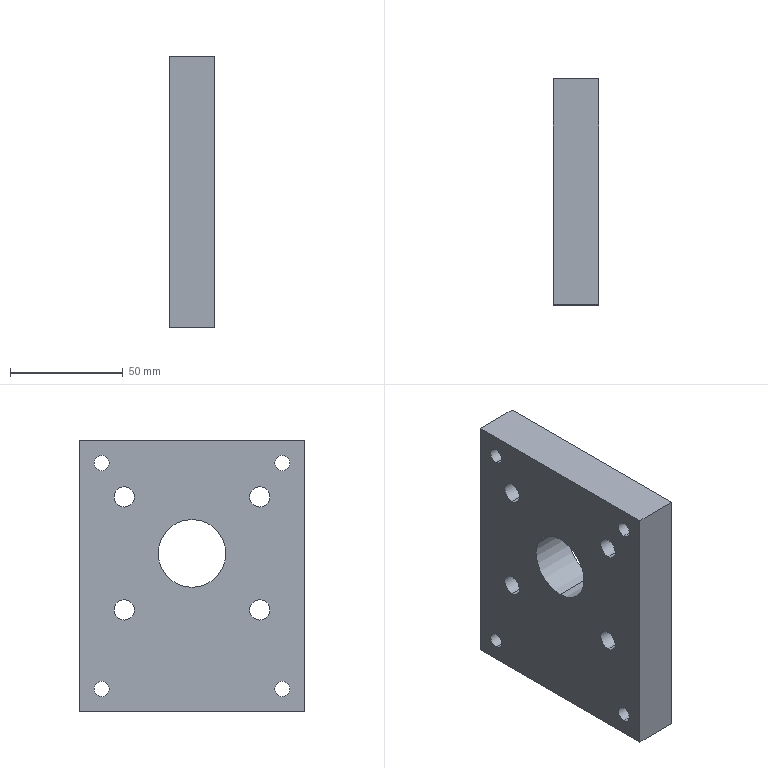Part | SolidWorks | features HoleWzd 2, Extrusion 1, ICE 1 | 1 solid | 36 faces | box 20 x 100 x 120 mm | volume 213797 mm3 | cylinder 26 | plane 10 | commonest cylinder face diameters 6.8 x8 9 x8 15 x8 30 x2
STEP:
#1=CARTESIAN_POINT('',(0.,40.,53.4));
#2=VERTEX_POINT('',#1);
#3=CARTESIAN_POINT('',(0.,40.,46.6));
#4=VERTEX_POINT('',#3);
#5=CARTESIAN_POINT('',(0.,40.,50.));
#6=DIRECTION('',(1.,0.,0.));
#7=DIRECTION('',(0.,0.,-1.));
#8=AXIS2_PLACEMENT_3D('',#5,#6,#7);
#9=CIRCLE('',#8,3.4);
#10=EDGE_CURVE('',#2,#4,#9,.T.);
#11=ORIENTED_EDGE('',*,*,#10,.F.);
#12=CARTESIAN_POINT('',(20.,40.,53.4));
#13=VERTEX_POINT('',#12);
#14=CARTESIAN_POINT('',(20.,40.,53.4));
#15=DIRECTION('',(1.,0.,0.));
#16=VECTOR('',#15,1000.);
#17=LINE('',#14,#16);
#18=EDGE_CURVE('',#2,#13,#17,.T.);
#19=ORIENTED_EDGE('',*,*,#18,.T.);
#20=CARTESIAN_POINT('',(20.,40.,46.6));
#21=VERTEX_POINT('',#20);
#22=CARTESIAN_POINT('',(20.,40.,50.));
#23=DIRECTION('',(1.,0.,0.));
#24=DIRECTION('',(0.,0.,-1.));
#25=AXIS2_PLACEMENT_3D('',#22,#23,#24);
#26=CIRCLE('',#25,3.4);
#27=EDGE_CURVE('',#13,#21,#26,.T.);
#28=ORIENTED_EDGE('',*,*,#27,.T.);
#29=CARTESIAN_POINT('',(20.,40.,46.6));
#30=DIRECTION('',(1.,0.,0.));
#31=VECTOR('',#30,1000.);
#32=LINE('',#29,#31);
#33=EDGE_CURVE('',#4,#21,#32,.T.);
#34=ORIENTED_EDGE('',*,*,#33,.F.);
#35=EDGE_LOOP('',(#11,#19,#28,#34));
#36=FACE_OUTER_BOUND('',#35,.T.);
#37=CARTESIAN_POINT('',(20.,40.,50.));
#38=DIRECTION('',(1.,0.,0.));
#39=DIRECTION('',(0.,0.,-1.));
#40=AXIS2_PLACEMENT_3D('',#37,#38,#39);
#41=CYLINDRICAL_SURFACE('',#40,3.4);
#42=ADVANCED_FACE('',(#36),#41,.F.);
#43=CARTESIAN_POINT('',(0.,-40.,53.4));
#44=VERTEX_POINT('',#43);
#45=CARTESIAN_POINT('',(0.,-40.,46.6));
#46=VERTEX_POINT('',#45);
#47=CARTESIAN_POINT('',(0.,-40.,50.));
#48=DIRECTION('',(1.,0.,0.));
#49=DIRECTION('',(0.,0.,-1.));
#50=AXIS2_PLACEMENT_3D('',#47,#48,#49);
#51=CIRCLE('',#50,3.4);
#52=EDGE_CURVE('',#44,#46,#51,.T.);
#53=ORIENTED_EDGE('',*,*,#52,.F.);
#54=CARTESIAN_POINT('',(20.,-40.,53.4));
#55=VERTEX_POINT('',#54);
#56=CARTESIAN_POINT('',(20.,-40.,53.4));
#57=DIRECTION('',(1.,0.,0.));
#58=VECTOR('',#57,1000.);
#59=LINE('',#56,#58);
#60=EDGE_CURVE('',#44,#55,#59,.T.);
#61=ORIENTED_EDGE('',*,*,#60,.T.);
#62=CARTESIAN_POINT('',(20.,-40.,46.6));
#63=VERTEX_POINT('',#62);
#64=CARTESIAN_POINT('',(20.,-40.,50.));
#65=DIRECTION('',(1.,0.,0.));
#66=DIRECTION('',(0.,0.,-1.));
#67=AXIS2_PLACEMENT_3D('',#64,#65,#66);
#68=CIRCLE('',#67,3.4);
#69=EDGE_CURVE('',#55,#63,#68,.T.);
#70=ORIENTED_EDGE('',*,*,#69,.T.);
#71=CARTESIAN_POINT('',(20.,-40.,46.6));
#72=DIRECTION('',(1.,0.,0.));
#73=VECTOR('',#72,1000.);
#74=LINE('',#71,#73);
#75=EDGE_CURVE('',#46,#63,#74,.T.);
#76=ORIENTED_EDGE('',*,*,#75,.F.);
#77=EDGE_LOOP('',(#53,#61,#70,#76));
#78=FACE_OUTER_BOUND('',#77,.T.);
#79=CARTESIAN_POINT('',(20.,-40.,50.));
#80=DIRECTION('',(1.,0.,0.));
#81=DIRECTION('',(0.,0.,-1.));
#82=AXIS2_PLACEMENT_3D('',#79,#80,#81);
#83=CYLINDRICAL_SURFACE('',#82,3.4);
#84=ADVANCED_FACE('',(#78),#83,.F.);
#85=CARTESIAN_POINT('',(0.,-40.,-46.6));
#86=VERTEX_POINT('',#85);
#87=CARTESIAN_POINT('',(0.,-40.,-53.4));
#88=VERTEX_POINT('',#87);
#89=CARTESIAN_POINT('',(0.,-40.,-50.));
#90=DIRECTION('',(1.,0.,0.));
#91=DIRECTION('',(0.,0.,-1.));
#92=AXIS2_PLACEMENT_3D('',#89,#90,#91);
#93=CIRCLE('',#92,3.4);
#94=EDGE_CURVE('',#86,#88,#93,.T.);
#95=ORIENTED_EDGE('',*,*,#94,.F.);
#96=CARTESIAN_POINT('',(20.,-40.,-46.6));
#97=VERTEX_POINT('',#96);
#98=CARTESIAN_POINT('',(20.,-40.,-46.6));
#99=DIRECTION('',(1.,0.,0.));
#100=VECTOR('',#99,1000.);
#101=LINE('',#98,#100);
#102=EDGE_CURVE('',#86,#97,#101,.T.);
#103=ORIENTED_EDGE('',*,*,#102,.T.);
#104=CARTESIAN_POINT('',(20.,-40.,-53.4));
#105=VERTEX_POINT('',#104);
#106=CARTESIAN_POINT('',(20.,-40.,-50.));
#107=DIRECTION('',(1.,0.,0.));
#108=DIRECTION('',(0.,0.,-1.));
#109=AXIS2_PLACEMENT_3D('',#106,#107,#108);
#110=CIRCLE('',#109,3.4);
#111=EDGE_CURVE('',#97,#105,#110,.T.);
#112=ORIENTED_EDGE('',*,*,#111,.T.);
#113=CARTESIAN_POINT('',(20.,-40.,-53.4));
#114=DIRECTION('',(1.,0.,0.));
#115=VECTOR('',#114,1000.);
#116=LINE('',#113,#115);
#117=EDGE_CURVE('',#88,#105,#116,.T.);
#118=ORIENTED_EDGE('',*,*,#117,.F.);
#119=EDGE_LOOP('',(#95,#103,#112,#118));
#120=FACE_OUTER_BOUND('',#119,.T.);
#121=CARTESIAN_POINT('',(20.,-40.,-50.));
#122=DIRECTION('',(1.,0.,0.));
#123=DIRECTION('',(0.,0.,-1.));
#124=AXIS2_PLACEMENT_3D('',#121,#122,#123);
#125=CYLINDRICAL_SURFACE('',#124,3.4);
#126=ADVANCED_FACE('',(#120),#125,.F.);
#127=CARTESIAN_POINT('',(0.,40.,-46.6));
#128=VERTEX_POINT('',#127);
#129=CARTESIAN_POINT('',(0.,40.,-53.4));
#130=VERTEX_POINT('',#129);
#131=CARTESIAN_POINT('',(0.,40.,-50.));
#132=DIRECTION('',(1.,0.,0.));
#133=DIRECTION('',(0.,0.,-1.));
#134=AXIS2_PLACEMENT_3D('',#131,#132,#133);
#135=CIRCLE('',#134,3.4);
#136=EDGE_CURVE('',#128,#130,#135,.T.);
#137=ORIENTED_EDGE('',*,*,#136,.F.);
#138=CARTESIAN_POINT('',(20.,40.,-46.6));
#139=VERTEX_POINT('',#138);
#140=CARTESIAN_POINT('',(20.,40.,-46.6));
#141=DIRECTION('',(1.,0.,0.));
#142=VECTOR('',#141,1000.);
#143=LINE('',#140,#142);
#144=EDGE_CURVE('',#128,#139,#143,.T.);
#145=ORIENTED_EDGE('',*,*,#144,.T.);
#146=CARTESIAN_POINT('',(20.,40.,-53.4));
#147=VERTEX_POINT('',#146);
#148=CARTESIAN_POINT('',(20.,40.,-50.));
#149=DIRECTION('',(1.,0.,0.));
#150=DIRECTION('',(0.,0.,-1.));
#151=AXIS2_PLACEMENT_3D('',#148,#149,#150);
#152=CIRCLE('',#151,3.4);
#153=EDGE_CURVE('',#139,#147,#152,.T.);
#154=ORIENTED_EDGE('',*,*,#153,.T.);
#155=CARTESIAN_POINT('',(20.,40.,-53.4));
#156=DIRECTION('',(1.,0.,0.));
#157=VECTOR('',#156,1000.);
#158=LINE('',#155,#157);
#159=EDGE_CURVE('',#130,#147,#158,.T.);
#160=ORIENTED_EDGE('',*,*,#159,.F.);
#161=EDGE_LOOP('',(#137,#145,#154,#160));
#162=FACE_OUTER_BOUND('',#161,.T.);
#163=CARTESIAN_POINT('',(20.,40.,-50.));
#164=DIRECTION('',(1.,0.,0.));
#165=DIRECTION('',(0.,0.,-1.));
#166=AXIS2_PLACEMENT_3D('',#163,#164,#165);
#167=CYLINDRICAL_SURFACE('',#166,3.4);
#168=ADVANCED_FACE('',(#162),#167,.F.);
#169=CARTESIAN_POINT('',(0.,0.,25.));
#170=VERTEX_POINT('',#169);
#171=CARTESIAN_POINT('',(0.,0.,-5.));
#172=VERTEX_POINT('',#171);
#173=CARTESIAN_POINT('',(0.,0.,10.));
#174=DIRECTION('',(1.,0.,0.));
#175=DIRECTION('',(0.,0.,-1.));
#176=AXIS2_PLACEMENT_3D('',#173,#174,#175);
#177=CIRCLE('',#176,15.);
#178=EDGE_CURVE('',#170,#172,#177,.T.);
#179=ORIENTED_EDGE('',*,*,#178,.F.);
#180=CARTESIAN_POINT('',(20.,0.,25.));
#181=VERTEX_POINT('',#180);
#182=CARTESIAN_POINT('',(0.,0.,25.));
#183=DIRECTION('',(1.,0.,0.));
#184=VECTOR('',#183,1000.);
#185=LINE('',#182,#184);
#186=EDGE_CURVE('',#170,#181,#185,.T.);
#187=ORIENTED_EDGE('',*,*,#186,.T.);
#188=CARTESIAN_POINT('',(20.,0.,-5.));
#189=VERTEX_POINT('',#188);
#190=CARTESIAN_POINT('',(20.,0.,10.));
#191=DIRECTION('',(1.,0.,0.));
#192=DIRECTION('',(0.,0.,-1.));
#193=AXIS2_PLACEMENT_3D('',#190,#191,#192);
#194=CIRCLE('',#193,15.);
#195=EDGE_CURVE('',#181,#189,#194,.T.);
#196=ORIENTED_EDGE('',*,*,#195,.T.);
#197=CARTESIAN_POINT('',(0.,0.,-5.));
#198=DIRECTION('',(1.,0.,0.));
#199=VECTOR('',#198,1000.);
#200=LINE('',#197,#199);
#201=EDGE_CURVE('',#172,#189,#200,.T.);
#202=ORIENTED_EDGE('',*,*,#201,.F.);
#203=EDGE_LOOP('',(#179,#187,#196,#202));
#204=FACE_OUTER_BOUND('',#203,.T.);
#205=CARTESIAN_POINT('',(0.,0.,10.));
#206=DIRECTION('',(1.,0.,0.));
#207=DIRECTION('',(0.,0.,-1.));
#208=AXIS2_PLACEMENT_3D('',#205,#206,#207);
#209=CYLINDRICAL_SURFACE('',#208,15.);
#210=ADVANCED_FACE('',(#204),#209,.F.);
#211=CARTESIAN_POINT('',(11.,30.,42.5));
#212=VERTEX_POINT('',#211);
#213=CARTESIAN_POINT('',(11.,30.,27.5));
#214=VERTEX_POINT('',#213);
#215=CARTESIAN_POINT('',(11.,30.,35.));
#216=DIRECTION('',(1.,0.,0.));
#217=DIRECTION('',(0.,0.,-1.));
#218=AXIS2_PLACEMENT_3D('',#215,#216,#217);
#219=CIRCLE('',#218,7.5);
#220=EDGE_CURVE('',#212,#214,#219,.T.);
#221=ORIENTED_EDGE('',*,*,#220,.F.);
#222=CARTESIAN_POINT('',(20.,30.,42.5));
#223=VERTEX_POINT('',#222);
#224=CARTESIAN_POINT('',(20.,30.,42.5));
#225=DIRECTION('',(1.,0.,0.));
#226=VECTOR('',#225,1000.);
#227=LINE('',#224,#226);
#228=EDGE_CURVE('',#212,#223,#227,.T.);
#229=ORIENTED_EDGE('',*,*,#228,.T.);
#230=CARTESIAN_POINT('',(20.,30.,27.5));
#231=VERTEX_POINT('',#230);
#232=CARTESIAN_POINT('',(20.,30.,35.));
#233=DIRECTION('',(1.,0.,0.));
#234=DIRECTION('',(0.,0.,-1.));
#235=AXIS2_PLACEMENT_3D('',#232,#233,#234);
#236=CIRCLE('',#235,7.5);
#237=EDGE_CURVE('',#223,#231,#236,.T.);
#238=ORIENTED_EDGE('',*,*,#237,.T.);
#239=CARTESIAN_POINT('',(20.,30.,27.5));
#240=DIRECTION('',(1.,0.,0.));
#241=VECTOR('',#240,1000.);
#242=LINE('',#239,#241);
#243=EDGE_CURVE('',#214,#231,#242,.T.);
#244=ORIENTED_EDGE('',*,*,#243,.F.);
#245=EDGE_LOOP('',(#221,#229,#238,#244));
#246=FACE_OUTER_BOUND('',#245,.T.);
#247=CARTESIAN_POINT('',(20.,30.,35.));
#248=DIRECTION('',(1.,0.,0.));
#249=DIRECTION('',(0.,0.,-1.));
#250=AXIS2_PLACEMENT_3D('',#247,#248,#249);
#251=CYLINDRICAL_SURFACE('',#250,7.5);
#252=ADVANCED_FACE('',(#246),#251,.F.);
#253=CARTESIAN_POINT('',(0.,30.,39.5));
#254=VERTEX_POINT('',#253);
#255=CARTESIAN_POINT('',(0.,30.,30.5));
#256=VERTEX_POINT('',#255);
#257=CARTESIAN_POINT('',(0.,30.,35.));
#258=DIRECTION('',(1.,0.,0.));
#259=DIRECTION('',(0.,0.,-1.));
#260=AXIS2_PLACEMENT_3D('',#257,#258,#259);
#261=CIRCLE('',#260,4.5);
#262=EDGE_CURVE('',#254,#256,#261,.T.);
#263=ORIENTED_EDGE('',*,*,#262,.F.);
#264=CARTESIAN_POINT('',(11.,30.,39.5));
#265=VERTEX_POINT('',#264);
#266=CARTESIAN_POINT('',(20.,30.,39.5));
#267=DIRECTION('',(1.,0.,0.));
#268=VECTOR('',#267,1000.);
#269=LINE('',#266,#268);
#270=EDGE_CURVE('',#254,#265,#269,.T.);
#271=ORIENTED_EDGE('',*,*,#270,.T.);
#272=CARTESIAN_POINT('',(11.,30.,30.5));
#273=VERTEX_POINT('',#272);
#274=CARTESIAN_POINT('',(11.,30.,35.));
#275=DIRECTION('',(1.,0.,0.));
#276=DIRECTION('',(0.,0.,-1.));
#277=AXIS2_PLACEMENT_3D('',#274,#275,#276);
#278=CIRCLE('',#277,4.5);
#279=EDGE_CURVE('',#265,#273,#278,.T.);
#280=ORIENTED_EDGE('',*,*,#279,.T.);
#281=CARTESIAN_POINT('',(20.,30.,30.5));
#282=DIRECTION('',(1.,0.,0.));
#283=VECTOR('',#282,1000.);
#284=LINE('',#281,#283);
#285=EDGE_CURVE('',#256,#273,#284,.T.);
#286=ORIENTED_EDGE('',*,*,#285,.F.);
#287=EDGE_LOOP('',(#263,#271,#280,#286));
#288=FACE_OUTER_BOUND('',#287,.T.);
#289=CARTESIAN_POINT('',(20.,30.,35.));
#290=DIRECTION('',(1.,0.,0.));
#291=DIRECTION('',(0.,0.,-1.));
#292=AXIS2_PLACEMENT_3D('',#289,#290,#291);
#293=CYLINDRICAL_SURFACE('',#292,4.5);
#294=ADVANCED_FACE('',(#288),#293,.F.);
#295=CARTESIAN_POINT('',(11.,30.,-7.5));
#296=VERTEX_POINT('',#295);
#297=CARTESIAN_POINT('',(11.,30.,-22.5));
#298=VERTEX_POINT('',#297);
#299=CARTESIAN_POINT('',(11.,30.,-15.));
#300=DIRECTION('',(1.,0.,0.));
#301=DIRECTION('',(0.,0.,-1.));
#302=AXIS2_PLACEMENT_3D('',#299,#300,#301);
#303=CIRCLE('',#302,7.5);
#304=EDGE_CURVE('',#296,#298,#303,.T.);
#305=ORIENTED_EDGE('',*,*,#304,.F.);
#306=CARTESIAN_POINT('',(20.,30.,-7.5));
#307=VERTEX_POINT('',#306);
#308=CARTESIAN_POINT('',(20.,30.,-7.5));
#309=DIRECTION('',(1.,0.,0.));
#310=VECTOR('',#309,1000.);
#311=LINE('',#308,#310);
#312=EDGE_CURVE('',#296,#307,#311,.T.);
#313=ORIENTED_EDGE('',*,*,#312,.T.);
#314=CARTESIAN_POINT('',(20.,30.,-22.5));
#315=VERTEX_POINT('',#314);
#316=CARTESIAN_POINT('',(20.,30.,-15.));
#317=DIRECTION('',(1.,0.,0.));
#318=DIRECTION('',(0.,0.,-1.));
#319=AXIS2_PLACEMENT_3D('',#316,#317,#318);
#320=CIRCLE('',#319,7.5);
#321=EDGE_CURVE('',#307,#315,#320,.T.);
#322=ORIENTED_EDGE('',*,*,#321,.T.);
#323=CARTESIAN_POINT('',(20.,30.,-22.5));
#324=DIRECTION('',(1.,0.,0.));
#325=VECTOR('',#324,1000.);
#326=LINE('',#323,#325);
#327=EDGE_CURVE('',#298,#315,#326,.T.);
#328=ORIENTED_EDGE('',*,*,#327,.F.);
#329=EDGE_LOOP('',(#305,#313,#322,#328));
#330=FACE_OUTER_BOUND('',#329,.T.);
#331=CARTESIAN_POINT('',(20.,30.,-15.));
#332=DIRECTION('',(1.,0.,0.));
#333=DIRECTION('',(0.,0.,-1.));
#334=AXIS2_PLACEMENT_3D('',#331,#332,#333);
#335=CYLINDRICAL_SURFACE('',#334,7.5);
#336=ADVANCED_FACE('',(#330),#335,.F.);
#337=CARTESIAN_POINT('',(0.,30.,-10.5));
#338=VERTEX_POINT('',#337);
#339=CARTESIAN_POINT('',(0.,30.,-19.5));
#340=VERTEX_POINT('',#339);
#341=CARTESIAN_POINT('',(0.,30.,-15.));
#342=DIRECTION('',(1.,0.,0.));
#343=DIRECTION('',(0.,0.,-1.));
#344=AXIS2_PLACEMENT_3D('',#341,#342,#343);
#345=CIRCLE('',#344,4.5);
#346=EDGE_CURVE('',#338,#340,#345,.T.);
#347=ORIENTED_EDGE('',*,*,#346,.F.);
#348=CARTESIAN_POINT('',(11.,30.,-10.5));
#349=VERTEX_POINT('',#348);
#350=CARTESIAN_POINT('',(20.,30.,-10.5));
#351=DIRECTION('',(1.,0.,0.));
#352=VECTOR('',#351,1000.);
#353=LINE('',#350,#352);
#354=EDGE_CURVE('',#338,#349,#353,.T.);
#355=ORIENTED_EDGE('',*,*,#354,.T.);
#356=CARTESIAN_POINT('',(11.,30.,-19.5));
#357=VERTEX_POINT('',#356);
#358=CARTESIAN_POINT('',(11.,30.,-15.));
#359=DIRECTION('',(1.,0.,0.));
#360=DIRECTION('',(0.,0.,-1.));
#361=AXIS2_PLACEMENT_3D('',#358,#359,#360);
#362=CIRCLE('',#361,4.5);
#363=EDGE_CURVE('',#349,#357,#362,.T.);
#364=ORIENTED_EDGE('',*,*,#363,.T.);
#365=CARTESIAN_POINT('',(20.,30.,-19.5));
#366=DIRECTION('',(1.,0.,0.));
#367=VECTOR('',#366,1000.);
#368=LINE('',#365,#367);
#369=EDGE_CURVE('',#340,#357,#368,.T.);
#370=ORIENTED_EDGE('',*,*,#369,.F.);
#371=EDGE_LOOP('',(#347,#355,#364,#370));
#372=FACE_OUTER_BOUND('',#371,.T.);
#373=CARTESIAN_POINT('',(20.,30.,-15.));
#374=DIRECTION('',(1.,0.,0.));
#375=DIRECTION('',(0.,0.,-1.));
#376=AXIS2_PLACEMENT_3D('',#373,#374,#375);
#377=CYLINDRICAL_SURFACE('',#376,4.5);
#378=ADVANCED_FACE('',(#372),#377,.F.);
#379=CARTESIAN_POINT('',(11.,-30.,42.5));
#380=VERTEX_POINT('',#379);
#381=CARTESIAN_POINT('',(11.,-30.,27.5));
#382=VERTEX_POINT('',#381);
#383=CARTESIAN_POINT('',(11.,-30.,35.));
#384=DIRECTION('',(1.,0.,0.));
#385=DIRECTION('',(0.,0.,-1.));
#386=AXIS2_PLACEMENT_3D('',#383,#384,#385);
#387=CIRCLE('',#386,7.5);
#388=EDGE_CURVE('',#380,#382,#387,.T.);
#389=ORIENTED_EDGE('',*,*,#388,.F.);
#390=CARTESIAN_POINT('',(20.,-30.,42.5));
#391=VERTEX_POINT('',#390);
#392=CARTESIAN_POINT('',(20.,-30.,42.5));
#393=DIRECTION('',(1.,0.,0.));
#394=VECTOR('',#393,1000.);
#395=LINE('',#392,#394);
#396=EDGE_CURVE('',#380,#391,#395,.T.);
#397=ORIENTED_EDGE('',*,*,#396,.T.);
#398=CARTESIAN_POINT('',(20.,-30.,27.5));
#399=VERTEX_POINT('',#398);
#400=CARTESIAN_POINT('',(20.,-30.,35.));
#401=DIRECTION('',(1.,0.,0.));
#402=DIRECTION('',(0.,0.,-1.));
#403=AXIS2_PLACEMENT_3D('',#400,#401,#402);
#404=CIRCLE('',#403,7.5);
#405=EDGE_CURVE('',#391,#399,#404,.T.);
#406=ORIENTED_EDGE('',*,*,#405,.T.);
#407=CARTESIAN_POINT('',(20.,-30.,27.5));
#408=DIRECTION('',(1.,0.,0.));
#409=VECTOR('',#408,1000.);
#410=LINE('',#407,#409);
#411=EDGE_CURVE('',#382,#399,#410,.T.);
#412=ORIENTED_EDGE('',*,*,#411,.F.);
#413=EDGE_LOOP('',(#389,#397,#406,#412));
#414=FACE_OUTER_BOUND('',#413,.T.);
#415=CARTESIAN_POINT('',(20.,-30.,35.));
#416=DIRECTION('',(1.,0.,0.));
#417=DIRECTION('',(0.,0.,-1.));
#418=AXIS2_PLACEMENT_3D('',#415,#416,#417);
#419=CYLINDRICAL_SURFACE('',#418,7.5);
#420=ADVANCED_FACE('',(#414),#419,.F.);
#421=CARTESIAN_POINT('',(0.,-30.,39.5));
#422=VERTEX_POINT('',#421);
#423=CARTESIAN_POINT('',(0.,-30.,30.5));
#424=VERTEX_POINT('',#423);
#425=CARTESIAN_POINT('',(0.,-30.,35.));
#426=DIRECTION('',(1.,0.,0.));
#427=DIRECTION('',(0.,0.,-1.));
#428=AXIS2_PLACEMENT_3D('',#425,#426,#427);
#429=CIRCLE('',#428,4.5);
#430=EDGE_CURVE('',#422,#424,#429,.T.);
#431=ORIENTED_EDGE('',*,*,#430,.F.);
#432=CARTESIAN_POINT('',(11.,-30.,39.5));
#433=VERTEX_POINT('',#432);
#434=CARTESIAN_POINT('',(20.,-30.,39.5));
#435=DIRECTION('',(1.,0.,0.));
#436=VECTOR('',#435,1000.);
#437=LINE('',#434,#436);
#438=EDGE_CURVE('',#422,#433,#437,.T.);
#439=ORIENTED_EDGE('',*,*,#438,.T.);
#440=CARTESIAN_POINT('',(11.,-30.,30.5));
#441=VERTEX_POINT('',#440);
#442=CARTESIAN_POINT('',(11.,-30.,35.));
#443=DIRECTION('',(1.,0.,0.));
#444=DIRECTION('',(0.,0.,-1.));
#445=AXIS2_PLACEMENT_3D('',#442,#443,#444);
#446=CIRCLE('',#445,4.5);
#447=EDGE_CURVE('',#433,#441,#446,.T.);
#448=ORIENTED_EDGE('',*,*,#447,.T.);
#449=CARTESIAN_POINT('',(20.,-30.,30.5));
#450=DIRECTION('',(1.,0.,0.));
#451=VECTOR('',#450,1000.);
#452=LINE('',#449,#451);
#453=EDGE_CURVE('',#424,#441,#452,.T.);
#454=ORIENTED_EDGE('',*,*,#453,.F.);
#455=EDGE_LOOP('',(#431,#439,#448,#454));
#456=FACE_OUTER_BOUND('',#455,.T.);
#457=CARTESIAN_POINT('',(20.,-30.,35.));
#458=DIRECTION('',(1.,0.,0.));
#459=DIRECTION('',(0.,0.,-1.));
#460=AXIS2_PLACEMENT_3D('',#457,#458,#459);
#461=CYLINDRICAL_SURFACE('',#460,4.5);
#462=ADVANCED_FACE('',(#456),#461,.F.);
#463=CARTESIAN_POINT('',(11.,-30.,-7.5));
#464=VERTEX_POINT('',#463);
#465=CARTESIAN_POINT('',(11.,-30.,-22.5));
#466=VERTEX_POINT('',#465);
#467=CARTESIAN_POINT('',(11.,-30.,-15.));
#468=DIRECTION('',(1.,0.,0.));
#469=DIRECTION('',(0.,0.,-1.));
#470=AXIS2_PLACEMENT_3D('',#467,#468,#469);
#471=CIRCLE('',#470,7.5);
#472=EDGE_CURVE('',#464,#466,#471,.T.);
#473=ORIENTED_EDGE('',*,*,#472,.F.);
#474=CARTESIAN_POINT('',(20.,-30.,-7.5));
#475=VERTEX_POINT('',#474);
#476=CARTESIAN_POINT('',(20.,-30.,-7.5));
#477=DIRECTION('',(1.,0.,0.));
#478=VECTOR('',#477,1000.);
#479=LINE('',#476,#478);
#480=EDGE_CURVE('',#464,#475,#479,.T.);
#481=ORIENTED_EDGE('',*,*,#480,.T.);
#482=CARTESIAN_POINT('',(20.,-30.,-22.5));
#483=VERTEX_POINT('',#482);
#484=CARTESIAN_POINT('',(20.,-30.,-15.));
#485=DIRECTION('',(1.,0.,0.));
#486=DIRECTION('',(0.,0.,-1.));
#487=AXIS2_PLACEMENT_3D('',#484,#485,#486);
#488=CIRCLE('',#487,7.5);
#489=EDGE_CURVE('',#475,#483,#488,.T.);
#490=ORIENTED_EDGE('',*,*,#489,.T.);
#491=CARTESIAN_POINT('',(20.,-30.,-22.5));
#492=DIRECTION('',(1.,0.,0.));
#493=VECTOR('',#492,1000.);
#494=LINE('',#491,#493);
#495=EDGE_CURVE('',#466,#483,#494,.T.);
#496=ORIENTED_EDGE('',*,*,#495,.F.);
#497=EDGE_LOOP('',(#473,#481,#490,#496));
#498=FACE_OUTER_BOUND('',#497,.T.);
#499=CARTESIAN_POINT('',(20.,-30.,-15.));
#500=DIRECTION('',(1.,0.,0.));
#501=DIRECTION('',(0.,0.,-1.));
#502=AXIS2_PLACEMENT_3D('',#499,#500,#501);
#503=CYLINDRICAL_SURFACE('',#502,7.5);
#504=ADVANCED_FACE('',(#498),#503,.F.);
#505=CARTESIAN_POINT('',(0.,-30.,-10.5));
#506=VERTEX_POINT('',#505);
#507=CARTESIAN_POINT('',(0.,-30.,-19.5));
#508=VERTEX_POINT('',#507);
#509=CARTESIAN_POINT('',(0.,-30.,-15.));
#510=DIRECTION('',(1.,0.,0.));
#511=DIRECTION('',(0.,0.,-1.));
#512=AXIS2_PLACEMENT_3D('',#509,#510,#511);
#513=CIRCLE('',#512,4.5);
#514=EDGE_CURVE('',#506,#508,#513,.T.);
#515=ORIENTED_EDGE('',*,*,#514,.F.);
#516=CARTESIAN_POINT('',(11.,-30.,-10.5));
#517=VERTEX_POINT('',#516);
#518=CARTESIAN_POINT('',(20.,-30.,-10.5));
#519=DIRECTION('',(1.,0.,0.));
#520=VECTOR('',#519,1000.);
#521=LINE('',#518,#520);
#522=EDGE_CURVE('',#506,#517,#521,.T.);
#523=ORIENTED_EDGE('',*,*,#522,.T.);
#524=CARTESIAN_POINT('',(11.,-30.,-19.5));
#525=VERTEX_POINT('',#524);
#526=CARTESIAN_POINT('',(11.,-30.,-15.));
#527=DIRECTION('',(1.,0.,0.));
#528=DIRECTION('',(0.,0.,-1.));
#529=AXIS2_PLACEMENT_3D('',#526,#527,#528);
#530=CIRCLE('',#529,4.5);
#531=EDGE_CURVE('',#517,#525,#530,.T.);
#532=ORIENTED_EDGE('',*,*,#531,.T.);
#533=CARTESIAN_POINT('',(20.,-30.,-19.5));
#534=DIRECTION('',(1.,0.,0.));
#535=VECTOR('',#534,1000.);
#536=LINE('',#533,#535);
#537=EDGE_CURVE('',#508,#525,#536,.T.);
#538=ORIENTED_EDGE('',*,*,#537,.F.);
#539=EDGE_LOOP('',(#515,#523,#532,#538));
#540=FACE_OUTER_BOUND('',#539,.T.);
#541=CARTESIAN_POINT('',(20.,-30.,-15.));
#542=DIRECTION('',(1.,0.,0.));
#543=DIRECTION('',(0.,0.,-1.));
#544=AXIS2_PLACEMENT_3D('',#541,#542,#543);
#545=CYLINDRICAL_SURFACE('',#544,4.5);
#546=ADVANCED_FACE('',(#540),#545,.F.);
#547=CARTESIAN_POINT('',(0.,-50.,-60.));
#548=VERTEX_POINT('',#547);
#549=CARTESIAN_POINT('',(0.,50.,-60.));
#550=VERTEX_POINT('',#549);
#551=CARTESIAN_POINT('',(0.,50.,-60.));
#552=DIRECTION('',(0.,1.,0.));
#553=VECTOR('',#552,1000.);
#554=LINE('',#551,#553);
#555=EDGE_CURVE('',#548,#550,#554,.T.);
#556=ORIENTED_EDGE('',*,*,#555,.T.);
#557=CARTESIAN_POINT('',(20.,50.,-60.));
#558=VERTEX_POINT('',#557);
#559=CARTESIAN_POINT('',(20.,50.,-60.));
#560=DIRECTION('',(-1.,0.,0.));
#561=VECTOR('',#560,1000.);
#562=LINE('',#559,#561);
#563=EDGE_CURVE('',#558,#550,#562,.T.);
#564=ORIENTED_EDGE('',*,*,#563,.F.);
#565=CARTESIAN_POINT('',(20.,-50.,-60.));
#566=VERTEX_POINT('',#565);
#567=CARTESIAN_POINT('',(20.,50.,-60.));
#568=DIRECTION('',(0.,1.,0.));
#569=VECTOR('',#568,1000.);
#570=LINE('',#567,#569);
#571=EDGE_CURVE('',#566,#558,#570,.T.);
#572=ORIENTED_EDGE('',*,*,#571,.F.);
#573=CARTESIAN_POINT('',(20.,-50.,-60.));
#574=DIRECTION('',(-1.,0.,0.));
#575=VECTOR('',#574,1000.);
#576=LINE('',#573,#575);
#577=EDGE_CURVE('',#566,#548,#576,.T.);
#578=ORIENTED_EDGE('',*,*,#577,.T.);
#579=EDGE_LOOP('',(#556,#564,#572,#578));
#580=FACE_OUTER_BOUND('',#579,.T.);
#581=CARTESIAN_POINT('',(20.,50.,-60.));
#582=DIRECTION('',(0.,0.,1.));
#583=DIRECTION('',(0.,-1.,0.));
#584=AXIS2_PLACEMENT_3D('',#581,#582,#583);
#585=PLANE('',#584);
#586=ADVANCED_FACE('',(#580),#585,.F.);
#587=CARTESIAN_POINT('',(0.,50.,60.));
#588=VERTEX_POINT('',#587);
#589=CARTESIAN_POINT('',(0.,50.,60.));
#590=DIRECTION('',(0.,0.,1.));
#591=VECTOR('',#590,1000.);
#592=LINE('',#589,#591);
#593=EDGE_CURVE('',#550,#588,#592,.T.);
#594=ORIENTED_EDGE('',*,*,#593,.T.);
#595=CARTESIAN_POINT('',(20.,50.,60.));
#596=VERTEX_POINT('',#595);
#597=CARTESIAN_POINT('',(20.,50.,60.));
#598=DIRECTION('',(-1.,0.,0.));
#599=VECTOR('',#598,1000.);
#600=LINE('',#597,#599);
#601=EDGE_CURVE('',#596,#588,#600,.T.);
#602=ORIENTED_EDGE('',*,*,#601,.F.);
#603=CARTESIAN_POINT('',(20.,50.,60.));
#604=DIRECTION('',(0.,0.,1.));
#605=VECTOR('',#604,1000.);
#606=LINE('',#603,#605);
#607=EDGE_CURVE('',#558,#596,#606,.T.);
#608=ORIENTED_EDGE('',*,*,#607,.F.);
#609=ORIENTED_EDGE('',*,*,#563,.T.);
#610=EDGE_LOOP('',(#594,#602,#608,#609));
#611=FACE_OUTER_BOUND('',#610,.T.);
#612=CARTESIAN_POINT('',(20.,50.,60.));
#613=DIRECTION('',(0.,-1.,0.));
#614=DIRECTION('',(0.,0.,-1.));
#615=AXIS2_PLACEMENT_3D('',#612,#613,#614);
#616=PLANE('',#615);
#617=ADVANCED_FACE('',(#611),#616,.F.);
#618=CARTESIAN_POINT('',(0.,-50.,60.));
#619=VERTEX_POINT('',#618);
#620=CARTESIAN_POINT('',(0.,50.,60.));
#621=DIRECTION('',(0.,-1.,0.));
#622=VECTOR('',#621,1000.);
#623=LINE('',#620,#622);
#624=EDGE_CURVE('',#588,#619,#623,.T.);
#625=ORIENTED_EDGE('',*,*,#624,.T.);
#626=CARTESIAN_POINT('',(20.,-50.,60.));
#627=VERTEX_POINT('',#626);
#628=CARTESIAN_POINT('',(20.,-50.,60.));
#629=DIRECTION('',(-1.,0.,0.));
#630=VECTOR('',#629,1000.);
#631=LINE('',#628,#630);
#632=EDGE_CURVE('',#627,#619,#631,.T.);
#633=ORIENTED_EDGE('',*,*,#632,.F.);
#634=CARTESIAN_POINT('',(20.,50.,60.));
#635=DIRECTION('',(0.,-1.,0.));
#636=VECTOR('',#635,1000.);
#637=LINE('',#634,#636);
#638=EDGE_CURVE('',#596,#627,#637,.T.);
#639=ORIENTED_EDGE('',*,*,#638,.F.);
#640=ORIENTED_EDGE('',*,*,#601,.T.);
#641=EDGE_LOOP('',(#625,#633,#639,#640));
#642=FACE_OUTER_BOUND('',#641,.T.);
#643=CARTESIAN_POINT('',(20.,50.,60.));
#644=DIRECTION('',(0.,0.,-1.));
#645=DIRECTION('',(0.,1.,0.));
#646=AXIS2_PLACEMENT_3D('',#643,#644,#645);
#647=PLANE('',#646);
#648=ADVANCED_FACE('',(#642),#647,.F.);
#649=CARTESIAN_POINT('',(0.,-50.,60.));
#650=DIRECTION('',(0.,0.,-1.));
#651=VECTOR('',#650,1000.);
#652=LINE('',#649,#651);
#653=EDGE_CURVE('',#619,#548,#652,.T.);
#654=ORIENTED_EDGE('',*,*,#653,.T.);
#655=ORIENTED_EDGE('',*,*,#577,.F.);
#656=CARTESIAN_POINT('',(20.,-50.,60.));
#657=DIRECTION('',(0.,0.,-1.));
#658=VECTOR('',#657,1000.);
#659=LINE('',#656,#658);
#660=EDGE_CURVE('',#627,#566,#659,.T.);
#661=ORIENTED_EDGE('',*,*,#660,.F.);
#662=ORIENTED_EDGE('',*,*,#632,.T.);
#663=EDGE_LOOP('',(#654,#655,#661,#662));
#664=FACE_OUTER_BOUND('',#663,.T.);
#665=CARTESIAN_POINT('',(20.,-50.,60.));
#666=DIRECTION('',(0.,1.,0.));
#667=DIRECTION('',(0.,0.,1.));
#668=AXIS2_PLACEMENT_3D('',#665,#666,#667);
#669=PLANE('',#668);
#670=ADVANCED_FACE('',(#664),#669,.F.);
#671=CARTESIAN_POINT('',(20.,40.,50.));
#672=DIRECTION('',(1.,0.,0.));
#673=DIRECTION('',(0.,0.,-1.));
#674=AXIS2_PLACEMENT_3D('',#671,#672,#673);
#675=CIRCLE('',#674,3.4);
#676=EDGE_CURVE('',#21,#13,#675,.T.);
#677=ORIENTED_EDGE('',*,*,#676,.F.);
#678=ORIENTED_EDGE('',*,*,#27,.F.);
#679=EDGE_LOOP('',(#677,#678));
#680=FACE_BOUND('',#679,.T.);
#681=CARTESIAN_POINT('',(20.,-40.,50.));
#682=DIRECTION('',(1.,0.,0.));
#683=DIRECTION('',(0.,0.,-1.));
#684=AXIS2_PLACEMENT_3D('',#681,#682,#683);
#685=CIRCLE('',#684,3.4);
#686=EDGE_CURVE('',#63,#55,#685,.T.);
#687=ORIENTED_EDGE('',*,*,#686,.F.);
#688=ORIENTED_EDGE('',*,*,#69,.F.);
#689=EDGE_LOOP('',(#687,#688));
#690=FACE_BOUND('',#689,.T.);
#691=CARTESIAN_POINT('',(20.,-40.,-50.));
#692=DIRECTION('',(1.,0.,0.));
#693=DIRECTION('',(0.,0.,-1.));
#694=AXIS2_PLACEMENT_3D('',#691,#692,#693);
#695=CIRCLE('',#694,3.4);
#696=EDGE_CURVE('',#105,#97,#695,.T.);
#697=ORIENTED_EDGE('',*,*,#696,.F.);
#698=ORIENTED_EDGE('',*,*,#111,.F.);
#699=EDGE_LOOP('',(#697,#698));
#700=FACE_BOUND('',#699,.T.);
#701=CARTESIAN_POINT('',(20.,40.,-50.));
#702=DIRECTION('',(1.,0.,0.));
#703=DIRECTION('',(0.,0.,-1.));
#704=AXIS2_PLACEMENT_3D('',#701,#702,#703);
#705=CIRCLE('',#704,3.4);
#706=EDGE_CURVE('',#147,#139,#705,.T.);
#707=ORIENTED_EDGE('',*,*,#706,.F.);
#708=ORIENTED_EDGE('',*,*,#153,.F.);
#709=EDGE_LOOP('',(#707,#708));
#710=FACE_BOUND('',#709,.T.);
#711=CARTESIAN_POINT('',(20.,0.,10.));
#712=DIRECTION('',(1.,0.,0.));
#713=DIRECTION('',(0.,0.,-1.));
#714=AXIS2_PLACEMENT_3D('',#711,#712,#713);
#715=CIRCLE('',#714,15.);
#716=EDGE_CURVE('',#189,#181,#715,.T.);
#717=ORIENTED_EDGE('',*,*,#716,.F.);
#718=ORIENTED_EDGE('',*,*,#195,.F.);
#719=EDGE_LOOP('',(#717,#718));
#720=FACE_BOUND('',#719,.T.);
#721=CARTESIAN_POINT('',(20.,30.,35.));
#722=DIRECTION('',(1.,0.,0.));
#723=DIRECTION('',(0.,0.,-1.));
#724=AXIS2_PLACEMENT_3D('',#721,#722,#723);
#725=CIRCLE('',#724,7.5);
#726=EDGE_CURVE('',#231,#223,#725,.T.);
#727=ORIENTED_EDGE('',*,*,#726,.F.);
#728=ORIENTED_EDGE('',*,*,#237,.F.);
#729=EDGE_LOOP('',(#727,#728));
#730=FACE_BOUND('',#729,.T.);
#731=CARTESIAN_POINT('',(20.,30.,-15.));
#732=DIRECTION('',(1.,0.,0.));
#733=DIRECTION('',(0.,0.,-1.));
#734=AXIS2_PLACEMENT_3D('',#731,#732,#733);
#735=CIRCLE('',#734,7.5);
#736=EDGE_CURVE('',#315,#307,#735,.T.);
#737=ORIENTED_EDGE('',*,*,#736,.F.);
#738=ORIENTED_EDGE('',*,*,#321,.F.);
#739=EDGE_LOOP('',(#737,#738));
#740=FACE_BOUND('',#739,.T.);
#741=CARTESIAN_POINT('',(20.,-30.,35.));
#742=DIRECTION('',(1.,0.,0.));
#743=DIRECTION('',(0.,0.,-1.));
#744=AXIS2_PLACEMENT_3D('',#741,#742,#743);
#745=CIRCLE('',#744,7.5);
#746=EDGE_CURVE('',#399,#391,#745,.T.);
#747=ORIENTED_EDGE('',*,*,#746,.F.);
#748=ORIENTED_EDGE('',*,*,#405,.F.);
#749=EDGE_LOOP('',(#747,#748));
#750=FACE_BOUND('',#749,.T.);
#751=CARTESIAN_POINT('',(20.,-30.,-15.));
#752=DIRECTION('',(1.,0.,0.));
#753=DIRECTION('',(0.,0.,-1.));
#754=AXIS2_PLACEMENT_3D('',#751,#752,#753);
#755=CIRCLE('',#754,7.5);
#756=EDGE_CURVE('',#483,#475,#755,.T.);
#757=ORIENTED_EDGE('',*,*,#756,.F.);
#758=ORIENTED_EDGE('',*,*,#489,.F.);
#759=EDGE_LOOP('',(#757,#758));
#760=FACE_BOUND('',#759,.T.);
#761=ORIENTED_EDGE('',*,*,#571,.T.);
#762=ORIENTED_EDGE('',*,*,#607,.T.);
#763=ORIENTED_EDGE('',*,*,#638,.T.);
#764=ORIENTED_EDGE('',*,*,#660,.T.);
#765=EDGE_LOOP('',(#761,#762,#763,#764));
#766=FACE_OUTER_BOUND('',#765,.T.);
#767=CARTESIAN_POINT('',(20.,0.,0.));
#768=DIRECTION('',(1.,0.,0.));
#769=DIRECTION('',(0.,0.,-1.));
#770=AXIS2_PLACEMENT_3D('',#767,#768,#769);
#771=PLANE('',#770);
#772=ADVANCED_FACE('',(#680,#690,#700,#710,#720,#730,#740,#750,#760,#766),#771,.T.);
#773=CARTESIAN_POINT('',(0.,40.,50.));
#774=DIRECTION('',(1.,0.,0.));
#775=DIRECTION('',(0.,0.,-1.));
#776=AXIS2_PLACEMENT_3D('',#773,#774,#775);
#777=CIRCLE('',#776,3.4);
#778=EDGE_CURVE('',#4,#2,#777,.T.);
#779=ORIENTED_EDGE('',*,*,#778,.T.);
#780=ORIENTED_EDGE('',*,*,#10,.T.);
#781=EDGE_LOOP('',(#779,#780));
#782=FACE_BOUND('',#781,.T.);
#783=CARTESIAN_POINT('',(0.,-40.,50.));
#784=DIRECTION('',(1.,0.,0.));
#785=DIRECTION('',(0.,0.,-1.));
#786=AXIS2_PLACEMENT_3D('',#783,#784,#785);
#787=CIRCLE('',#786,3.4);
#788=EDGE_CURVE('',#46,#44,#787,.T.);
#789=ORIENTED_EDGE('',*,*,#788,.T.);
#790=ORIENTED_EDGE('',*,*,#52,.T.);
#791=EDGE_LOOP('',(#789,#790));
#792=FACE_BOUND('',#791,.T.);
#793=CARTESIAN_POINT('',(0.,-40.,-50.));
#794=DIRECTION('',(1.,0.,0.));
#795=DIRECTION('',(0.,0.,-1.));
#796=AXIS2_PLACEMENT_3D('',#793,#794,#795);
#797=CIRCLE('',#796,3.4);
#798=EDGE_CURVE('',#88,#86,#797,.T.);
#799=ORIENTED_EDGE('',*,*,#798,.T.);
#800=ORIENTED_EDGE('',*,*,#94,.T.);
#801=EDGE_LOOP('',(#799,#800));
#802=FACE_BOUND('',#801,.T.);
#803=CARTESIAN_POINT('',(0.,40.,-50.));
#804=DIRECTION('',(1.,0.,0.));
#805=DIRECTION('',(0.,0.,-1.));
#806=AXIS2_PLACEMENT_3D('',#803,#804,#805);
#807=CIRCLE('',#806,3.4);
#808=EDGE_CURVE('',#130,#128,#807,.T.);
#809=ORIENTED_EDGE('',*,*,#808,.T.);
#810=ORIENTED_EDGE('',*,*,#136,.T.);
#811=EDGE_LOOP('',(#809,#810));
#812=FACE_BOUND('',#811,.T.);
#813=CARTESIAN_POINT('',(0.,0.,10.));
#814=DIRECTION('',(1.,0.,0.));
#815=DIRECTION('',(0.,0.,-1.));
#816=AXIS2_PLACEMENT_3D('',#813,#814,#815);
#817=CIRCLE('',#816,15.);
#818=EDGE_CURVE('',#172,#170,#817,.T.);
#819=ORIENTED_EDGE('',*,*,#818,.T.);
#820=ORIENTED_EDGE('',*,*,#178,.T.);
#821=EDGE_LOOP('',(#819,#820));
#822=FACE_BOUND('',#821,.T.);
#823=CARTESIAN_POINT('',(0.,30.,35.));
#824=DIRECTION('',(1.,0.,0.));
#825=DIRECTION('',(0.,0.,-1.));
#826=AXIS2_PLACEMENT_3D('',#823,#824,#825);
#827=CIRCLE('',#826,4.5);
#828=EDGE_CURVE('',#256,#254,#827,.T.);
#829=ORIENTED_EDGE('',*,*,#828,.T.);
#830=ORIENTED_EDGE('',*,*,#262,.T.);
#831=EDGE_LOOP('',(#829,#830));
#832=FACE_BOUND('',#831,.T.);
#833=CARTESIAN_POINT('',(0.,30.,-15.));
#834=DIRECTION('',(1.,0.,0.));
#835=DIRECTION('',(0.,0.,-1.));
#836=AXIS2_PLACEMENT_3D('',#833,#834,#835);
#837=CIRCLE('',#836,4.5);
#838=EDGE_CURVE('',#340,#338,#837,.T.);
#839=ORIENTED_EDGE('',*,*,#838,.T.);
#840=ORIENTED_EDGE('',*,*,#346,.T.);
#841=EDGE_LOOP('',(#839,#840));
#842=FACE_BOUND('',#841,.T.);
#843=CARTESIAN_POINT('',(0.,-30.,35.));
#844=DIRECTION('',(1.,0.,0.));
#845=DIRECTION('',(0.,0.,-1.));
#846=AXIS2_PLACEMENT_3D('',#843,#844,#845);
#847=CIRCLE('',#846,4.5);
#848=EDGE_CURVE('',#424,#422,#847,.T.);
#849=ORIENTED_EDGE('',*,*,#848,.T.);
#850=ORIENTED_EDGE('',*,*,#430,.T.);
#851=EDGE_LOOP('',(#849,#850));
#852=FACE_BOUND('',#851,.T.);
#853=CARTESIAN_POINT('',(0.,-30.,-15.));
#854=DIRECTION('',(1.,0.,0.));
#855=DIRECTION('',(0.,0.,-1.));
#856=AXIS2_PLACEMENT_3D('',#853,#854,#855);
#857=CIRCLE('',#856,4.5);
#858=EDGE_CURVE('',#508,#506,#857,.T.);
#859=ORIENTED_EDGE('',*,*,#858,.T.);
#860=ORIENTED_EDGE('',*,*,#514,.T.);
#861=EDGE_LOOP('',(#859,#860));
#862=FACE_BOUND('',#861,.T.);
#863=ORIENTED_EDGE('',*,*,#555,.F.);
#864=ORIENTED_EDGE('',*,*,#653,.F.);
#865=ORIENTED_EDGE('',*,*,#624,.F.);
#866=ORIENTED_EDGE('',*,*,#593,.F.);
#867=EDGE_LOOP('',(#863,#864,#865,#866));
#868=FACE_OUTER_BOUND('',#867,.T.);
#869=CARTESIAN_POINT('',(0.,0.,0.));
#870=DIRECTION('',(1.,0.,0.));
#871=DIRECTION('',(0.,0.,-1.));
#872=AXIS2_PLACEMENT_3D('',#869,#870,#871);
#873=PLANE('',#872);
#874=ADVANCED_FACE('',(#782,#792,#802,#812,#822,#832,#842,#852,#862,#868),#873,.F.);
#875=ORIENTED_EDGE('',*,*,#522,.F.);
#876=ORIENTED_EDGE('',*,*,#858,.F.);
#877=ORIENTED_EDGE('',*,*,#537,.T.);
#878=CARTESIAN_POINT('',(11.,-30.,-15.));
#879=DIRECTION('',(1.,0.,0.));
#880=DIRECTION('',(0.,0.,-1.));
#881=AXIS2_PLACEMENT_3D('',#878,#879,#880);
#882=CIRCLE('',#881,4.5);
#883=EDGE_CURVE('',#525,#517,#882,.T.);
#884=ORIENTED_EDGE('',*,*,#883,.T.);
#885=EDGE_LOOP('',(#875,#876,#877,#884));
#886=FACE_OUTER_BOUND('',#885,.T.);
#887=CARTESIAN_POINT('',(20.,-30.,-15.));
#888=DIRECTION('',(1.,0.,0.));
#889=DIRECTION('',(0.,0.,-1.));
#890=AXIS2_PLACEMENT_3D('',#887,#888,#889);
#891=CYLINDRICAL_SURFACE('',#890,4.5);
#892=ADVANCED_FACE('',(#886),#891,.F.);
#893=ORIENTED_EDGE('',*,*,#883,.F.);
#894=ORIENTED_EDGE('',*,*,#531,.F.);
#895=EDGE_LOOP('',(#893,#894));
#896=FACE_BOUND('',#895,.T.);
#897=CARTESIAN_POINT('',(11.,-30.,-15.));
#898=DIRECTION('',(1.,0.,0.));
#899=DIRECTION('',(0.,0.,-1.));
#900=AXIS2_PLACEMENT_3D('',#897,#898,#899);
#901=CIRCLE('',#900,7.5);
#902=EDGE_CURVE('',#466,#464,#901,.T.);
#903=ORIENTED_EDGE('',*,*,#902,.T.);
#904=ORIENTED_EDGE('',*,*,#472,.T.);
#905=EDGE_LOOP('',(#903,#904));
#906=FACE_OUTER_BOUND('',#905,.T.);
#907=CARTESIAN_POINT('',(11.,-25.5,-15.));
#908=DIRECTION('',(-1.,0.,0.));
#909=DIRECTION('',(0.,0.,1.));
#910=AXIS2_PLACEMENT_3D('',#907,#908,#909);
#911=PLANE('',#910);
#912=ADVANCED_FACE('',(#896,#906),#911,.F.);
#913=ORIENTED_EDGE('',*,*,#480,.F.);
#914=ORIENTED_EDGE('',*,*,#902,.F.);
#915=ORIENTED_EDGE('',*,*,#495,.T.);
#916=ORIENTED_EDGE('',*,*,#756,.T.);
#917=EDGE_LOOP('',(#913,#914,#915,#916));
#918=FACE_OUTER_BOUND('',#917,.T.);
#919=CARTESIAN_POINT('',(20.,-30.,-15.));
#920=DIRECTION('',(1.,0.,0.));
#921=DIRECTION('',(0.,0.,-1.));
#922=AXIS2_PLACEMENT_3D('',#919,#920,#921);
#923=CYLINDRICAL_SURFACE('',#922,7.5);
#924=ADVANCED_FACE('',(#918),#923,.F.);
#925=ORIENTED_EDGE('',*,*,#438,.F.);
#926=ORIENTED_EDGE('',*,*,#848,.F.);
#927=ORIENTED_EDGE('',*,*,#453,.T.);
#928=CARTESIAN_POINT('',(11.,-30.,35.));
#929=DIRECTION('',(1.,0.,0.));
#930=DIRECTION('',(0.,0.,-1.));
#931=AXIS2_PLACEMENT_3D('',#928,#929,#930);
#932=CIRCLE('',#931,4.5);
#933=EDGE_CURVE('',#441,#433,#932,.T.);
#934=ORIENTED_EDGE('',*,*,#933,.T.);
#935=EDGE_LOOP('',(#925,#926,#927,#934));
#936=FACE_OUTER_BOUND('',#935,.T.);
#937=CARTESIAN_POINT('',(20.,-30.,35.));
#938=DIRECTION('',(1.,0.,0.));
#939=DIRECTION('',(0.,0.,-1.));
#940=AXIS2_PLACEMENT_3D('',#937,#938,#939);
#941=CYLINDRICAL_SURFACE('',#940,4.5);
#942=ADVANCED_FACE('',(#936),#941,.F.);
#943=ORIENTED_EDGE('',*,*,#933,.F.);
#944=ORIENTED_EDGE('',*,*,#447,.F.);
#945=EDGE_LOOP('',(#943,#944));
#946=FACE_BOUND('',#945,.T.);
#947=CARTESIAN_POINT('',(11.,-30.,35.));
#948=DIRECTION('',(1.,0.,0.));
#949=DIRECTION('',(0.,0.,-1.));
#950=AXIS2_PLACEMENT_3D('',#947,#948,#949);
#951=CIRCLE('',#950,7.5);
#952=EDGE_CURVE('',#382,#380,#951,.T.);
#953=ORIENTED_EDGE('',*,*,#952,.T.);
#954=ORIENTED_EDGE('',*,*,#388,.T.);
#955=EDGE_LOOP('',(#953,#954));
#956=FACE_OUTER_BOUND('',#955,.T.);
#957=CARTESIAN_POINT('',(11.,-25.5,35.));
#958=DIRECTION('',(-1.,0.,0.));
#959=DIRECTION('',(0.,0.,1.));
#960=AXIS2_PLACEMENT_3D('',#957,#958,#959);
#961=PLANE('',#960);
#962=ADVANCED_FACE('',(#946,#956),#961,.F.);
#963=ORIENTED_EDGE('',*,*,#396,.F.);
#964=ORIENTED_EDGE('',*,*,#952,.F.);
#965=ORIENTED_EDGE('',*,*,#411,.T.);
#966=ORIENTED_EDGE('',*,*,#746,.T.);
#967=EDGE_LOOP('',(#963,#964,#965,#966));
#968=FACE_OUTER_BOUND('',#967,.T.);
#969=CARTESIAN_POINT('',(20.,-30.,35.));
#970=DIRECTION('',(1.,0.,0.));
#971=DIRECTION('',(0.,0.,-1.));
#972=AXIS2_PLACEMENT_3D('',#969,#970,#971);
#973=CYLINDRICAL_SURFACE('',#972,7.5);
#974=ADVANCED_FACE('',(#968),#973,.F.);
#975=ORIENTED_EDGE('',*,*,#354,.F.);
#976=ORIENTED_EDGE('',*,*,#838,.F.);
#977=ORIENTED_EDGE('',*,*,#369,.T.);
#978=CARTESIAN_POINT('',(11.,30.,-15.));
#979=DIRECTION('',(1.,0.,0.));
#980=DIRECTION('',(0.,0.,-1.));
#981=AXIS2_PLACEMENT_3D('',#978,#979,#980);
#982=CIRCLE('',#981,4.5);
#983=EDGE_CURVE('',#357,#349,#982,.T.);
#984=ORIENTED_EDGE('',*,*,#983,.T.);
#985=EDGE_LOOP('',(#975,#976,#977,#984));
#986=FACE_OUTER_BOUND('',#985,.T.);
#987=CARTESIAN_POINT('',(20.,30.,-15.));
#988=DIRECTION('',(1.,0.,0.));
#989=DIRECTION('',(0.,0.,-1.));
#990=AXIS2_PLACEMENT_3D('',#987,#988,#989);
#991=CYLINDRICAL_SURFACE('',#990,4.5);
#992=ADVANCED_FACE('',(#986),#991,.F.);
#993=ORIENTED_EDGE('',*,*,#983,.F.);
#994=ORIENTED_EDGE('',*,*,#363,.F.);
#995=EDGE_LOOP('',(#993,#994));
#996=FACE_BOUND('',#995,.T.);
#997=CARTESIAN_POINT('',(11.,30.,-15.));
#998=DIRECTION('',(1.,0.,0.));
#999=DIRECTION('',(0.,0.,-1.));
#1000=AXIS2_PLACEMENT_3D('',#997,#998,#999);
#1001=CIRCLE('',#1000,7.5);
#1002=EDGE_CURVE('',#298,#296,#1001,.T.);
#1003=ORIENTED_EDGE('',*,*,#1002,.T.);
#1004=ORIENTED_EDGE('',*,*,#304,.T.);
#1005=EDGE_LOOP('',(#1003,#1004));
#1006=FACE_OUTER_BOUND('',#1005,.T.);
#1007=CARTESIAN_POINT('',(11.,34.5,-15.));
#1008=DIRECTION('',(-1.,0.,0.));
#1009=DIRECTION('',(0.,0.,1.));
#1010=AXIS2_PLACEMENT_3D('',#1007,#1008,#1009);
#1011=PLANE('',#1010);
#1012=ADVANCED_FACE('',(#996,#1006),#1011,.F.);
#1013=ORIENTED_EDGE('',*,*,#312,.F.);
#1014=ORIENTED_EDGE('',*,*,#1002,.F.);
#1015=ORIENTED_EDGE('',*,*,#327,.T.);
#1016=ORIENTED_EDGE('',*,*,#736,.T.);
#1017=EDGE_LOOP('',(#1013,#1014,#1015,#1016));
#1018=FACE_OUTER_BOUND('',#1017,.T.);
#1019=CARTESIAN_POINT('',(20.,30.,-15.));
#1020=DIRECTION('',(1.,0.,0.));
#1021=DIRECTION('',(0.,0.,-1.));
#1022=AXIS2_PLACEMENT_3D('',#1019,#1020,#1021);
#1023=CYLINDRICAL_SURFACE('',#1022,7.5);
#1024=ADVANCED_FACE('',(#1018),#1023,.F.);
#1025=ORIENTED_EDGE('',*,*,#270,.F.);
#1026=ORIENTED_EDGE('',*,*,#828,.F.);
#1027=ORIENTED_EDGE('',*,*,#285,.T.);
#1028=CARTESIAN_POINT('',(11.,30.,35.));
#1029=DIRECTION('',(1.,0.,0.));
#1030=DIRECTION('',(0.,0.,-1.));
#1031=AXIS2_PLACEMENT_3D('',#1028,#1029,#1030);
#1032=CIRCLE('',#1031,4.5);
#1033=EDGE_CURVE('',#273,#265,#1032,.T.);
#1034=ORIENTED_EDGE('',*,*,#1033,.T.);
#1035=EDGE_LOOP('',(#1025,#1026,#1027,#1034));
#1036=FACE_OUTER_BOUND('',#1035,.T.);
#1037=CARTESIAN_POINT('',(20.,30.,35.));
#1038=DIRECTION('',(1.,0.,0.));
#1039=DIRECTION('',(0.,0.,-1.));
#1040=AXIS2_PLACEMENT_3D('',#1037,#1038,#1039);
#1041=CYLINDRICAL_SURFACE('',#1040,4.5);
#1042=ADVANCED_FACE('',(#1036),#1041,.F.);
#1043=ORIENTED_EDGE('',*,*,#1033,.F.);
#1044=ORIENTED_EDGE('',*,*,#279,.F.);
#1045=EDGE_LOOP('',(#1043,#1044));
#1046=FACE_BOUND('',#1045,.T.);
#1047=CARTESIAN_POINT('',(11.,30.,35.));
#1048=DIRECTION('',(1.,0.,0.));
#1049=DIRECTION('',(0.,0.,-1.));
#1050=AXIS2_PLACEMENT_3D('',#1047,#1048,#1049);
#1051=CIRCLE('',#1050,7.5);
#1052=EDGE_CURVE('',#214,#212,#1051,.T.);
#1053=ORIENTED_EDGE('',*,*,#1052,.T.);
#1054=ORIENTED_EDGE('',*,*,#220,.T.);
#1055=EDGE_LOOP('',(#1053,#1054));
#1056=FACE_OUTER_BOUND('',#1055,.T.);
#1057=CARTESIAN_POINT('',(11.,34.5,35.));
#1058=DIRECTION('',(-1.,0.,0.));
#1059=DIRECTION('',(0.,0.,1.));
#1060=AXIS2_PLACEMENT_3D('',#1057,#1058,#1059);
#1061=PLANE('',#1060);
#1062=ADVANCED_FACE('',(#1046,#1056),#1061,.F.);
#1063=ORIENTED_EDGE('',*,*,#228,.F.);
#1064=ORIENTED_EDGE('',*,*,#1052,.F.);
#1065=ORIENTED_EDGE('',*,*,#243,.T.);
#1066=ORIENTED_EDGE('',*,*,#726,.T.);
#1067=EDGE_LOOP('',(#1063,#1064,#1065,#1066));
#1068=FACE_OUTER_BOUND('',#1067,.T.);
#1069=CARTESIAN_POINT('',(20.,30.,35.));
#1070=DIRECTION('',(1.,0.,0.));
#1071=DIRECTION('',(0.,0.,-1.));
#1072=AXIS2_PLACEMENT_3D('',#1069,#1070,#1071);
#1073=CYLINDRICAL_SURFACE('',#1072,7.5);
#1074=ADVANCED_FACE('',(#1068),#1073,.F.);
#1075=ORIENTED_EDGE('',*,*,#186,.F.);
#1076=ORIENTED_EDGE('',*,*,#818,.F.);
#1077=ORIENTED_EDGE('',*,*,#201,.T.);
#1078=ORIENTED_EDGE('',*,*,#716,.T.);
#1079=EDGE_LOOP('',(#1075,#1076,#1077,#1078));
#1080=FACE_OUTER_BOUND('',#1079,.T.);
#1081=CARTESIAN_POINT('',(0.,0.,10.));
#1082=DIRECTION('',(1.,0.,0.));
#1083=DIRECTION('',(0.,0.,-1.));
#1084=AXIS2_PLACEMENT_3D('',#1081,#1082,#1083);
#1085=CYLINDRICAL_SURFACE('',#1084,15.);
#1086=ADVANCED_FACE('',(#1080),#1085,.F.);
#1087=ORIENTED_EDGE('',*,*,#144,.F.);
#1088=ORIENTED_EDGE('',*,*,#808,.F.);
#1089=ORIENTED_EDGE('',*,*,#159,.T.);
#1090=ORIENTED_EDGE('',*,*,#706,.T.);
#1091=EDGE_LOOP('',(#1087,#1088,#1089,#1090));
#1092=FACE_OUTER_BOUND('',#1091,.T.);
#1093=CARTESIAN_POINT('',(20.,40.,-50.));
#1094=DIRECTION('',(1.,0.,0.));
#1095=DIRECTION('',(0.,0.,-1.));
#1096=AXIS2_PLACEMENT_3D('',#1093,#1094,#1095);
#1097=CYLINDRICAL_SURFACE('',#1096,3.4);
#1098=ADVANCED_FACE('',(#1092),#1097,.F.);
#1099=ORIENTED_EDGE('',*,*,#102,.F.);
#1100=ORIENTED_EDGE('',*,*,#798,.F.);
#1101=ORIENTED_EDGE('',*,*,#117,.T.);
#1102=ORIENTED_EDGE('',*,*,#696,.T.);
#1103=EDGE_LOOP('',(#1099,#1100,#1101,#1102));
#1104=FACE_OUTER_BOUND('',#1103,.T.);
#1105=CARTESIAN_POINT('',(20.,-40.,-50.));
#1106=DIRECTION('',(1.,0.,0.));
#1107=DIRECTION('',(0.,0.,-1.));
#1108=AXIS2_PLACEMENT_3D('',#1105,#1106,#1107);
#1109=CYLINDRICAL_SURFACE('',#1108,3.4);
#1110=ADVANCED_FACE('',(#1104),#1109,.F.);
#1111=ORIENTED_EDGE('',*,*,#60,.F.);
#1112=ORIENTED_EDGE('',*,*,#788,.F.);
#1113=ORIENTED_EDGE('',*,*,#75,.T.);
#1114=ORIENTED_EDGE('',*,*,#686,.T.);
#1115=EDGE_LOOP('',(#1111,#1112,#1113,#1114));
#1116=FACE_OUTER_BOUND('',#1115,.T.);
#1117=CARTESIAN_POINT('',(20.,-40.,50.));
#1118=DIRECTION('',(1.,0.,0.));
#1119=DIRECTION('',(0.,0.,-1.));
#1120=AXIS2_PLACEMENT_3D('',#1117,#1118,#1119);
#1121=CYLINDRICAL_SURFACE('',#1120,3.4);
#1122=ADVANCED_FACE('',(#1116),#1121,.F.);
#1123=ORIENTED_EDGE('',*,*,#18,.F.);
#1124=ORIENTED_EDGE('',*,*,#778,.F.);
#1125=ORIENTED_EDGE('',*,*,#33,.T.);
#1126=ORIENTED_EDGE('',*,*,#676,.T.);
#1127=EDGE_LOOP('',(#1123,#1124,#1125,#1126));
#1128=FACE_OUTER_BOUND('',#1127,.T.);
#1129=CARTESIAN_POINT('',(20.,40.,50.));
#1130=DIRECTION('',(1.,0.,0.));
#1131=DIRECTION('',(0.,0.,-1.));
#1132=AXIS2_PLACEMENT_3D('',#1129,#1130,#1131);
#1133=CYLINDRICAL_SURFACE('',#1132,3.4);
#1134=ADVANCED_FACE('',(#1128),#1133,.F.);
#1135=CLOSED_SHELL('',(#42,#84,#126,#168,#210,#252,#294,#336,#378,#420,#462,#504,#546,#586,#617,#648,#670,#772,#874,#892,#912,#924,#942,#962,#974,#992,#1012,#1024,#1042,#1062,#1074,#1086,#1098,#1110,#1122,#1134));
#1136=MANIFOLD_SOLID_BREP('',#1135);
#1137=CARTESIAN_POINT('',(0.,0.,0.));
#1138=DIRECTION('',(0.,0.,1.));
#1139=DIRECTION('',(1.,0.,0.));
#1140=AXIS2_PLACEMENT_3D('',#1137,#1138,#1139);
#1141=(LENGTH_UNIT()NAMED_UNIT(*)SI_UNIT(.MILLI.,.METRE.));
#1142=UNCERTAINTY_MEASURE_WITH_UNIT(LENGTH_MEASURE(0.00001),#1141,'','');
#1143=(NAMED_UNIT(*)PLANE_ANGLE_UNIT()SI_UNIT($,.RADIAN.));
#1144=(NAMED_UNIT(*)SI_UNIT($,.STERADIAN.)SOLID_ANGLE_UNIT());
#1145=(GEOMETRIC_REPRESENTATION_CONTEXT(3)GLOBAL_UNCERTAINTY_ASSIGNED_CONTEXT((#1142))GLOBAL_UNIT_ASSIGNED_CONTEXT((#1141,#1143,#1144))REPRESENTATION_CONTEXT('',''));
#1146=ADVANCED_BREP_SHAPE_REPRESENTATION('',(#1136,#1140),#1145);